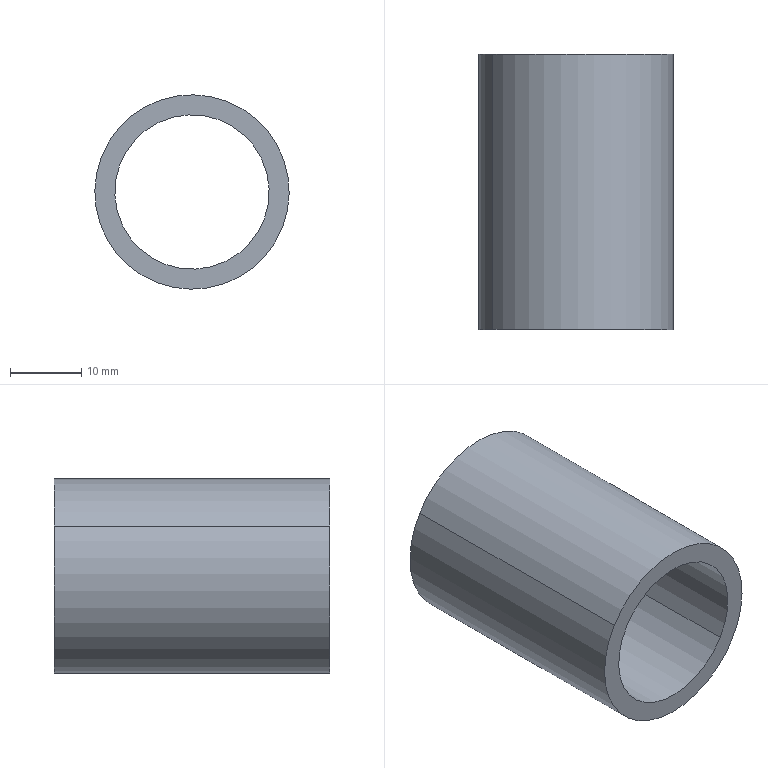Part | STEP file | [03]-12 | 1 solid | 6 faces | box 27.2 x 38.5 x 27.2 mm | volume 8263 mm3 | cylinder 4 | plane 2 | commonest cylinder face diameters 21.6 x2 27.2 x2
STEP:
#1=CARTESIAN_POINT('',(0.,0.,0.));
#2=DIRECTION('',(0.,0.,1.));
#3=DIRECTION('',(1.,0.,0.));
#4=AXIS2_PLACEMENT_3D('',#1,#2,#3);
#5=CARTESIAN_POINT('',(9.263,-20.,-5.553));
#6=VERTEX_POINT('',#5);
#7=CARTESIAN_POINT('',(9.263,18.5,-5.553));
#8=VERTEX_POINT('',#7);
#9=CARTESIAN_POINT('',(9.263,-20.,-5.553));
#10=DIRECTION('',(0.,1.,0.));
#11=VECTOR('',#10,1.);
#12=LINE('',#9,#11);
#13=CARTESIAN_POINT('',(0.,-20.,0.));
#14=DIRECTION('',(0.,1.,0.));
#15=DIRECTION('',(0.8577,0.,-0.5142));
#16=AXIS2_PLACEMENT_3D('',#13,#14,#15);
#17=CYLINDRICAL_SURFACE('',#16,10.8);
#18=CARTESIAN_POINT('',(6.283,0.));
#19=CARTESIAN_POINT('',(6.283,0.5833));
#20=CARTESIAN_POINT('',(6.283,1.75));
#21=CARTESIAN_POINT('',(6.283,3.5));
#22=CARTESIAN_POINT('',(6.283,5.25));
#23=CARTESIAN_POINT('',(6.283,7.));
#24=CARTESIAN_POINT('',(6.283,8.75));
#25=CARTESIAN_POINT('',(6.283,10.5));
#26=CARTESIAN_POINT('',(6.283,12.25));
#27=CARTESIAN_POINT('',(6.283,14.));
#28=CARTESIAN_POINT('',(6.283,15.75));
#29=CARTESIAN_POINT('',(6.283,17.5));
#30=CARTESIAN_POINT('',(6.283,19.25));
#31=CARTESIAN_POINT('',(6.283,21.));
#32=CARTESIAN_POINT('',(6.283,22.75));
#33=CARTESIAN_POINT('',(6.283,24.5));
#34=CARTESIAN_POINT('',(6.283,26.25));
#35=CARTESIAN_POINT('',(6.283,28.));
#36=CARTESIAN_POINT('',(6.283,29.75));
#37=CARTESIAN_POINT('',(6.283,31.5));
#38=CARTESIAN_POINT('',(6.283,33.25));
#39=CARTESIAN_POINT('',(6.283,35.));
#40=CARTESIAN_POINT('',(6.283,36.75));
#41=CARTESIAN_POINT('',(6.283,37.917));
#42=CARTESIAN_POINT('',(6.283,38.5));
#43=B_SPLINE_CURVE_WITH_KNOTS('',3,(#18,#19,#20,#21,#22,#23,#24,#25,#26,#27,#28,#29,#30,#31,#32,#33,#34,#35,#36,#37,#38,#39,#40,#41,#42),.UNSPECIFIED.,.F.,.F.,(4,1,1,1,1,1,1,1,1,1,1,1,1,1,1,1,1,1,1,1,1,1,4),(0.,1.75,3.5,5.25,7.,8.75,10.5,12.25,14.,15.75,17.5,19.25,21.,22.75,24.5,26.25,28.,29.75,31.5,33.25,35.,36.75,38.5),.QUASI_UNIFORM_KNOTS.);
#44=(GEOMETRIC_REPRESENTATION_CONTEXT(2)PARAMETRIC_REPRESENTATION_CONTEXT()REPRESENTATION_CONTEXT('',''));
#45=DEFINITIONAL_REPRESENTATION('',(#43),#44);
#46=PCURVE('',#17,#45);
#47=CARTESIAN_POINT('',(0.,-20.,0.));
#48=DIRECTION('',(0.,1.,0.));
#49=DIRECTION('',(0.8577,0.,-0.5142));
#50=AXIS2_PLACEMENT_3D('',#47,#48,#49);
#51=CYLINDRICAL_SURFACE('',#50,10.8);
#52=CARTESIAN_POINT('',(0.,0.));
#53=DIRECTION('',(0.,1.));
#54=VECTOR('',#53,1.);
#55=LINE('',#52,#54);
#56=(GEOMETRIC_REPRESENTATION_CONTEXT(2)PARAMETRIC_REPRESENTATION_CONTEXT()REPRESENTATION_CONTEXT('',''));
#57=DEFINITIONAL_REPRESENTATION('',(#55),#56);
#58=PCURVE('',#51,#57);
#59=SURFACE_CURVE('',#12,(#46,#58),.PCURVE_S1.);
#60=EDGE_CURVE('',#6,#8,#59,.T.);
#61=ORIENTED_EDGE('',*,*,#60,.T.);
#62=CARTESIAN_POINT('',(-9.263,18.5,5.553));
#63=VERTEX_POINT('',#62);
#64=CARTESIAN_POINT('',(0.,18.5,0.));
#65=DIRECTION('',(0.,1.,0.));
#66=DIRECTION('',(-0.8577,0.,0.5142));
#67=AXIS2_PLACEMENT_3D('',#64,#65,#66);
#68=CIRCLE('',#67,10.8);
#69=CARTESIAN_POINT('',(3.142,38.5));
#70=DIRECTION('',(1.,0.));
#71=VECTOR('',#70,1.);
#72=LINE('',#69,#71);
#73=(GEOMETRIC_REPRESENTATION_CONTEXT(2)PARAMETRIC_REPRESENTATION_CONTEXT()REPRESENTATION_CONTEXT('',''));
#74=DEFINITIONAL_REPRESENTATION('',(#72),#73);
#75=PCURVE('',#17,#74);
#76=CARTESIAN_POINT('',(0.,18.5,0.));
#77=DIRECTION('',(0.,1.,0.));
#78=DIRECTION('',(0.8577,0.,-0.5142));
#79=AXIS2_PLACEMENT_3D('',#76,#77,#78);
#80=PLANE('',#79);
#81=CARTESIAN_POINT('',(0.,0.));
#82=DIRECTION('',(-1.,0.));
#83=AXIS2_PLACEMENT_2D('',#81,#82);
#84=CIRCLE('',#83,10.8);
#85=(GEOMETRIC_REPRESENTATION_CONTEXT(2)PARAMETRIC_REPRESENTATION_CONTEXT()REPRESENTATION_CONTEXT('',''));
#86=DEFINITIONAL_REPRESENTATION('',(#84),#85);
#87=PCURVE('',#80,#86);
#88=SURFACE_CURVE('',#68,(#75,#87),.PCURVE_S1.);
#89=EDGE_CURVE('',#63,#8,#88,.T.);
#90=ORIENTED_EDGE('',*,*,#89,.F.);
#91=CARTESIAN_POINT('',(-9.263,-20.,5.553));
#92=VERTEX_POINT('',#91);
#93=CARTESIAN_POINT('',(-9.263,-20.,5.553));
#94=DIRECTION('',(0.,1.,0.));
#95=VECTOR('',#94,1.);
#96=LINE('',#93,#95);
#97=CARTESIAN_POINT('',(3.142,0.));
#98=DIRECTION('',(0.,1.));
#99=VECTOR('',#98,1.);
#100=LINE('',#97,#99);
#101=(GEOMETRIC_REPRESENTATION_CONTEXT(2)PARAMETRIC_REPRESENTATION_CONTEXT()REPRESENTATION_CONTEXT('',''));
#102=DEFINITIONAL_REPRESENTATION('',(#100),#101);
#103=PCURVE('',#17,#102);
#104=CARTESIAN_POINT('',(3.142,0.));
#105=DIRECTION('',(0.,1.));
#106=VECTOR('',#105,1.);
#107=LINE('',#104,#106);
#108=(GEOMETRIC_REPRESENTATION_CONTEXT(2)PARAMETRIC_REPRESENTATION_CONTEXT()REPRESENTATION_CONTEXT('',''));
#109=DEFINITIONAL_REPRESENTATION('',(#107),#108);
#110=PCURVE('',#51,#109);
#111=SURFACE_CURVE('',#96,(#103,#110),.PCURVE_S1.);
#112=EDGE_CURVE('',#92,#63,#111,.T.);
#113=ORIENTED_EDGE('',*,*,#112,.F.);
#114=CARTESIAN_POINT('',(0.,-20.,0.));
#115=DIRECTION('',(0.,-1.,0.));
#116=DIRECTION('',(0.8577,0.,-0.5142));
#117=AXIS2_PLACEMENT_3D('',#114,#115,#116);
#118=CIRCLE('',#117,10.8);
#119=CARTESIAN_POINT('',(6.283,0.));
#120=DIRECTION('',(-1.,0.));
#121=VECTOR('',#120,1.);
#122=LINE('',#119,#121);
#123=(GEOMETRIC_REPRESENTATION_CONTEXT(2)PARAMETRIC_REPRESENTATION_CONTEXT()REPRESENTATION_CONTEXT('',''));
#124=DEFINITIONAL_REPRESENTATION('',(#122),#123);
#125=PCURVE('',#17,#124);
#126=CARTESIAN_POINT('',(0.,-20.,0.));
#127=DIRECTION('',(0.,-1.,0.));
#128=DIRECTION('',(-0.8577,0.,0.5142));
#129=AXIS2_PLACEMENT_3D('',#126,#127,#128);
#130=PLANE('',#129);
#131=CARTESIAN_POINT('',(0.,0.));
#132=DIRECTION('',(-1.,0.));
#133=AXIS2_PLACEMENT_2D('',#131,#132);
#134=CIRCLE('',#133,10.8);
#135=(GEOMETRIC_REPRESENTATION_CONTEXT(2)PARAMETRIC_REPRESENTATION_CONTEXT()REPRESENTATION_CONTEXT('',''));
#136=DEFINITIONAL_REPRESENTATION('',(#134),#135);
#137=PCURVE('',#130,#136);
#138=SURFACE_CURVE('',#118,(#125,#137),.PCURVE_S1.);
#139=EDGE_CURVE('',#6,#92,#138,.T.);
#140=ORIENTED_EDGE('',*,*,#139,.F.);
#141=EDGE_LOOP('',(#61,#90,#113,#140));
#142=FACE_BOUND('',#141,.F.);
#143=ADVANCED_FACE('',(#142),#17,.F.);
#144=CARTESIAN_POINT('',(-11.665,-20.,6.993));
#145=VERTEX_POINT('',#144);
#146=CARTESIAN_POINT('',(11.665,-20.,-6.993));
#147=VERTEX_POINT('',#146);
#148=CARTESIAN_POINT('',(0.,-20.,0.));
#149=DIRECTION('',(0.,-1.,0.));
#150=DIRECTION('',(0.8577,0.,-0.5142));
#151=AXIS2_PLACEMENT_3D('',#148,#149,#150);
#152=CIRCLE('',#151,13.6);
#153=CARTESIAN_POINT('',(0.,-20.,0.));
#154=DIRECTION('',(0.,1.,0.));
#155=DIRECTION('',(0.8577,0.,-0.5142));
#156=AXIS2_PLACEMENT_3D('',#153,#154,#155);
#157=CYLINDRICAL_SURFACE('',#156,13.6);
#158=CARTESIAN_POINT('',(6.283,0.));
#159=DIRECTION('',(-1.,0.));
#160=VECTOR('',#159,1.);
#161=LINE('',#158,#160);
#162=(GEOMETRIC_REPRESENTATION_CONTEXT(2)PARAMETRIC_REPRESENTATION_CONTEXT()REPRESENTATION_CONTEXT('',''));
#163=DEFINITIONAL_REPRESENTATION('',(#161),#162);
#164=PCURVE('',#157,#163);
#165=CARTESIAN_POINT('',(0.,0.));
#166=DIRECTION('',(-1.,0.));
#167=AXIS2_PLACEMENT_2D('',#165,#166);
#168=CIRCLE('',#167,13.6);
#169=(GEOMETRIC_REPRESENTATION_CONTEXT(2)PARAMETRIC_REPRESENTATION_CONTEXT()REPRESENTATION_CONTEXT('',''));
#170=DEFINITIONAL_REPRESENTATION('',(#168),#169);
#171=PCURVE('',#130,#170);
#172=SURFACE_CURVE('',#152,(#164,#171),.PCURVE_S1.);
#173=EDGE_CURVE('',#145,#147,#172,.T.);
#174=ORIENTED_EDGE('',*,*,#173,.F.);
#175=CARTESIAN_POINT('',(-11.665,18.5,6.993));
#176=VERTEX_POINT('',#175);
#177=CARTESIAN_POINT('',(-11.665,-20.,6.993));
#178=DIRECTION('',(0.,1.,0.));
#179=VECTOR('',#178,1.);
#180=LINE('',#177,#179);
#181=CARTESIAN_POINT('',(3.142,0.));
#182=DIRECTION('',(0.,1.));
#183=VECTOR('',#182,1.);
#184=LINE('',#181,#183);
#185=(GEOMETRIC_REPRESENTATION_CONTEXT(2)PARAMETRIC_REPRESENTATION_CONTEXT()REPRESENTATION_CONTEXT('',''));
#186=DEFINITIONAL_REPRESENTATION('',(#184),#185);
#187=PCURVE('',#157,#186);
#188=CARTESIAN_POINT('',(0.,-20.,0.));
#189=DIRECTION('',(0.,1.,0.));
#190=DIRECTION('',(0.8577,0.,-0.5142));
#191=AXIS2_PLACEMENT_3D('',#188,#189,#190);
#192=CYLINDRICAL_SURFACE('',#191,13.6);
#193=CARTESIAN_POINT('',(3.142,0.));
#194=DIRECTION('',(0.,1.));
#195=VECTOR('',#194,1.);
#196=LINE('',#193,#195);
#197=(GEOMETRIC_REPRESENTATION_CONTEXT(2)PARAMETRIC_REPRESENTATION_CONTEXT()REPRESENTATION_CONTEXT('',''));
#198=DEFINITIONAL_REPRESENTATION('',(#196),#197);
#199=PCURVE('',#192,#198);
#200=SURFACE_CURVE('',#180,(#187,#199),.PCURVE_S1.);
#201=EDGE_CURVE('',#145,#176,#200,.T.);
#202=ORIENTED_EDGE('',*,*,#201,.T.);
#203=CARTESIAN_POINT('',(11.665,18.5,-6.993));
#204=VERTEX_POINT('',#203);
#205=CARTESIAN_POINT('',(0.,18.5,0.));
#206=DIRECTION('',(0.,1.,0.));
#207=DIRECTION('',(-0.8577,0.,0.5142));
#208=AXIS2_PLACEMENT_3D('',#205,#206,#207);
#209=CIRCLE('',#208,13.6);
#210=CARTESIAN_POINT('',(-3.142,38.5));
#211=DIRECTION('',(1.,0.));
#212=VECTOR('',#211,1.);
#213=LINE('',#210,#212);
#214=(GEOMETRIC_REPRESENTATION_CONTEXT(2)PARAMETRIC_REPRESENTATION_CONTEXT()REPRESENTATION_CONTEXT('',''));
#215=DEFINITIONAL_REPRESENTATION('',(#213),#214);
#216=PCURVE('',#157,#215);
#217=CARTESIAN_POINT('',(0.,0.));
#218=DIRECTION('',(-1.,0.));
#219=AXIS2_PLACEMENT_2D('',#217,#218);
#220=CIRCLE('',#219,13.6);
#221=(GEOMETRIC_REPRESENTATION_CONTEXT(2)PARAMETRIC_REPRESENTATION_CONTEXT()REPRESENTATION_CONTEXT('',''));
#222=DEFINITIONAL_REPRESENTATION('',(#220),#221);
#223=PCURVE('',#80,#222);
#224=SURFACE_CURVE('',#209,(#216,#223),.PCURVE_S1.);
#225=EDGE_CURVE('',#204,#176,#224,.T.);
#226=ORIENTED_EDGE('',*,*,#225,.F.);
#227=CARTESIAN_POINT('',(11.665,-20.,-6.993));
#228=DIRECTION('',(0.,1.,0.));
#229=VECTOR('',#228,1.);
#230=LINE('',#227,#229);
#231=CARTESIAN_POINT('',(0.,0.));
#232=DIRECTION('',(0.,1.));
#233=VECTOR('',#232,1.);
#234=LINE('',#231,#233);
#235=(GEOMETRIC_REPRESENTATION_CONTEXT(2)PARAMETRIC_REPRESENTATION_CONTEXT()REPRESENTATION_CONTEXT('',''));
#236=DEFINITIONAL_REPRESENTATION('',(#234),#235);
#237=PCURVE('',#157,#236);
#238=CARTESIAN_POINT('',(6.283,0.));
#239=DIRECTION('',(0.,1.));
#240=VECTOR('',#239,1.);
#241=LINE('',#238,#240);
#242=(GEOMETRIC_REPRESENTATION_CONTEXT(2)PARAMETRIC_REPRESENTATION_CONTEXT()REPRESENTATION_CONTEXT('',''));
#243=DEFINITIONAL_REPRESENTATION('',(#241),#242);
#244=PCURVE('',#192,#243);
#245=SURFACE_CURVE('',#230,(#237,#244),.PCURVE_S1.);
#246=EDGE_CURVE('',#147,#204,#245,.T.);
#247=ORIENTED_EDGE('',*,*,#246,.F.);
#248=EDGE_LOOP('',(#174,#202,#226,#247));
#249=FACE_BOUND('',#248,.T.);
#250=ADVANCED_FACE('',(#249),#157,.T.);
#251=CARTESIAN_POINT('',(0.,18.5,0.));
#252=DIRECTION('',(0.,1.,0.));
#253=DIRECTION('',(-0.8577,0.,0.5142));
#254=AXIS2_PLACEMENT_3D('',#251,#252,#253);
#255=CIRCLE('',#254,10.8);
#256=CARTESIAN_POINT('',(0.,0.));
#257=DIRECTION('',(-1.,0.));
#258=AXIS2_PLACEMENT_2D('',#256,#257);
#259=CIRCLE('',#258,10.8);
#260=(GEOMETRIC_REPRESENTATION_CONTEXT(2)PARAMETRIC_REPRESENTATION_CONTEXT()REPRESENTATION_CONTEXT('',''));
#261=DEFINITIONAL_REPRESENTATION('',(#259),#260);
#262=PCURVE('',#80,#261);
#263=CARTESIAN_POINT('',(-3.142,38.5));
#264=DIRECTION('',(1.,0.));
#265=VECTOR('',#264,1.);
#266=LINE('',#263,#265);
#267=(GEOMETRIC_REPRESENTATION_CONTEXT(2)PARAMETRIC_REPRESENTATION_CONTEXT()REPRESENTATION_CONTEXT('',''));
#268=DEFINITIONAL_REPRESENTATION('',(#266),#267);
#269=PCURVE('',#51,#268);
#270=SURFACE_CURVE('',#255,(#262,#269),.PCURVE_S1.);
#271=EDGE_CURVE('',#8,#63,#270,.T.);
#272=ORIENTED_EDGE('',*,*,#271,.F.);
#273=ORIENTED_EDGE('',*,*,#89,.F.);
#274=EDGE_LOOP('',(#272,#273));
#275=FACE_BOUND('',#274,.T.);
#276=ORIENTED_EDGE('',*,*,#225,.T.);
#277=CARTESIAN_POINT('',(0.,18.5,0.));
#278=DIRECTION('',(0.,1.,0.));
#279=DIRECTION('',(-0.8577,0.,0.5142));
#280=AXIS2_PLACEMENT_3D('',#277,#278,#279);
#281=CIRCLE('',#280,13.6);
#282=CARTESIAN_POINT('',(0.,0.));
#283=DIRECTION('',(-1.,0.));
#284=AXIS2_PLACEMENT_2D('',#282,#283);
#285=CIRCLE('',#284,13.6);
#286=(GEOMETRIC_REPRESENTATION_CONTEXT(2)PARAMETRIC_REPRESENTATION_CONTEXT()REPRESENTATION_CONTEXT('',''));
#287=DEFINITIONAL_REPRESENTATION('',(#285),#286);
#288=PCURVE('',#80,#287);
#289=CARTESIAN_POINT('',(3.142,38.5));
#290=DIRECTION('',(1.,0.));
#291=VECTOR('',#290,1.);
#292=LINE('',#289,#291);
#293=(GEOMETRIC_REPRESENTATION_CONTEXT(2)PARAMETRIC_REPRESENTATION_CONTEXT()REPRESENTATION_CONTEXT('',''));
#294=DEFINITIONAL_REPRESENTATION('',(#292),#293);
#295=PCURVE('',#192,#294);
#296=SURFACE_CURVE('',#281,(#288,#295),.PCURVE_S1.);
#297=EDGE_CURVE('',#176,#204,#296,.T.);
#298=ORIENTED_EDGE('',*,*,#297,.T.);
#299=EDGE_LOOP('',(#276,#298));
#300=FACE_BOUND('',#299,.T.);
#301=ADVANCED_FACE('',(#275,#300),#80,.T.);
#302=ORIENTED_EDGE('',*,*,#139,.F.);
#303=CARTESIAN_POINT('',(0.,-20.,0.));
#304=DIRECTION('',(0.,-1.,0.));
#305=DIRECTION('',(0.8577,0.,-0.5142));
#306=AXIS2_PLACEMENT_3D('',#303,#304,#305);
#307=CIRCLE('',#306,10.8);
#308=CARTESIAN_POINT('',(0.,0.));
#309=DIRECTION('',(-1.,0.));
#310=AXIS2_PLACEMENT_2D('',#308,#309);
#311=CIRCLE('',#310,10.8);
#312=(GEOMETRIC_REPRESENTATION_CONTEXT(2)PARAMETRIC_REPRESENTATION_CONTEXT()REPRESENTATION_CONTEXT('',''));
#313=DEFINITIONAL_REPRESENTATION('',(#311),#312);
#314=PCURVE('',#130,#313);
#315=CARTESIAN_POINT('',(6.283,0.));
#316=DIRECTION('',(-1.,0.));
#317=VECTOR('',#316,1.);
#318=LINE('',#315,#317);
#319=(GEOMETRIC_REPRESENTATION_CONTEXT(2)PARAMETRIC_REPRESENTATION_CONTEXT()REPRESENTATION_CONTEXT('',''));
#320=DEFINITIONAL_REPRESENTATION('',(#318),#319);
#321=PCURVE('',#51,#320);
#322=SURFACE_CURVE('',#307,(#314,#321),.PCURVE_S1.);
#323=EDGE_CURVE('',#92,#6,#322,.T.);
#324=ORIENTED_EDGE('',*,*,#323,.F.);
#325=EDGE_LOOP('',(#302,#324));
#326=FACE_BOUND('',#325,.T.);
#327=CARTESIAN_POINT('',(0.,-20.,0.));
#328=DIRECTION('',(0.,-1.,0.));
#329=DIRECTION('',(0.8577,0.,-0.5142));
#330=AXIS2_PLACEMENT_3D('',#327,#328,#329);
#331=CIRCLE('',#330,13.6);
#332=CARTESIAN_POINT('',(0.,0.));
#333=DIRECTION('',(-1.,0.));
#334=AXIS2_PLACEMENT_2D('',#332,#333);
#335=CIRCLE('',#334,13.6);
#336=(GEOMETRIC_REPRESENTATION_CONTEXT(2)PARAMETRIC_REPRESENTATION_CONTEXT()REPRESENTATION_CONTEXT('',''));
#337=DEFINITIONAL_REPRESENTATION('',(#335),#336);
#338=PCURVE('',#130,#337);
#339=CARTESIAN_POINT('',(6.283,0.));
#340=DIRECTION('',(-1.,0.));
#341=VECTOR('',#340,1.);
#342=LINE('',#339,#341);
#343=(GEOMETRIC_REPRESENTATION_CONTEXT(2)PARAMETRIC_REPRESENTATION_CONTEXT()REPRESENTATION_CONTEXT('',''));
#344=DEFINITIONAL_REPRESENTATION('',(#342),#343);
#345=PCURVE('',#192,#344);
#346=SURFACE_CURVE('',#331,(#338,#345),.PCURVE_S1.);
#347=EDGE_CURVE('',#147,#145,#346,.T.);
#348=ORIENTED_EDGE('',*,*,#347,.T.);
#349=ORIENTED_EDGE('',*,*,#173,.T.);
#350=EDGE_LOOP('',(#348,#349));
#351=FACE_BOUND('',#350,.T.);
#352=ADVANCED_FACE('',(#326,#351),#130,.T.);
#353=ORIENTED_EDGE('',*,*,#201,.F.);
#354=ORIENTED_EDGE('',*,*,#347,.F.);
#355=ORIENTED_EDGE('',*,*,#246,.T.);
#356=ORIENTED_EDGE('',*,*,#297,.F.);
#357=EDGE_LOOP('',(#353,#354,#355,#356));
#358=FACE_BOUND('',#357,.T.);
#359=ADVANCED_FACE('',(#358),#192,.T.);
#360=ORIENTED_EDGE('',*,*,#271,.F.);
#361=ORIENTED_EDGE('',*,*,#60,.F.);
#362=ORIENTED_EDGE('',*,*,#323,.F.);
#363=ORIENTED_EDGE('',*,*,#112,.T.);
#364=EDGE_LOOP('',(#360,#361,#362,#363));
#365=FACE_BOUND('',#364,.F.);
#366=ADVANCED_FACE('',(#365),#51,.F.);
#367=CLOSED_SHELL('',(#143,#250,#301,#352,#359,#366));
#368=MANIFOLD_SOLID_BREP('',#367);
#369=(LENGTH_UNIT()NAMED_UNIT(*)SI_UNIT(.MILLI.,.METRE.));
#370=UNCERTAINTY_MEASURE_WITH_UNIT(LENGTH_MEASURE(0.0000001),#369,'','');
#371=(NAMED_UNIT(*)PLANE_ANGLE_UNIT()SI_UNIT($,.RADIAN.));
#372=(NAMED_UNIT(*)SI_UNIT($,.STERADIAN.)SOLID_ANGLE_UNIT());
#373=(GEOMETRIC_REPRESENTATION_CONTEXT(3)GLOBAL_UNCERTAINTY_ASSIGNED_CONTEXT((#370))GLOBAL_UNIT_ASSIGNED_CONTEXT((#369,#371,#372))REPRESENTATION_CONTEXT('',''));
#374=ADVANCED_BREP_SHAPE_REPRESENTATION('',(#4,#368),#373);